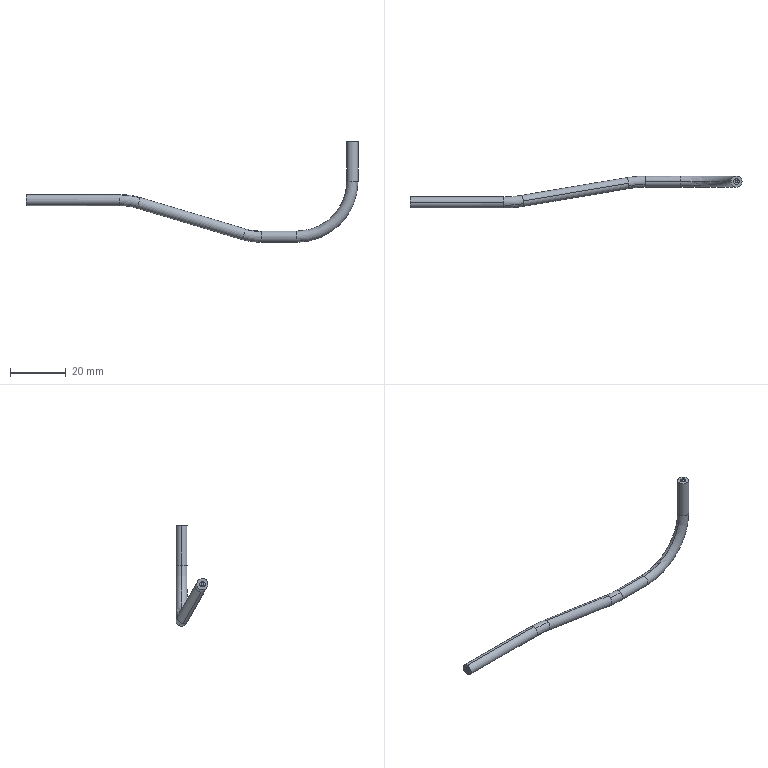Part | STEP file | [COMPANY_A Nylon 4-3 Copy] | 1 solid | 28 faces | box 119.5 x 11.5 x 36.167 mm | volume 1748 mm3 | cylinder 16 | torus 6 | plane 6 | commonest cylinder face diameters 4 x8 1 x4 2 x4
STEP:
#1=CARTESIAN_POINT('',(98.5,9.5,4.));
#2=VERTEX_POINT('',#1);
#3=CARTESIAN_POINT('',(98.5,9.5,0.));
#4=VERTEX_POINT('',#3);
#5=CARTESIAN_POINT('',(98.5,9.5,2.));
#6=DIRECTION('',(1.,0.,0.));
#7=DIRECTION('',(0.,-1.,0.));
#8=AXIS2_PLACEMENT_3D('',#5,#6,#7);
#9=CIRCLE('',#8,2.);
#10=EDGE_CURVE('',#2,#4,#9,.T.);
#11=ORIENTED_EDGE('',*,*,#10,.T.);
#12=CARTESIAN_POINT('',(120.5,9.5,22.));
#13=VERTEX_POINT('',#12);
#14=CARTESIAN_POINT('',(98.5,9.5,22.));
#15=DIRECTION('',(0.,-1.,0.));
#16=DIRECTION('',(1.,0.,0.));
#17=AXIS2_PLACEMENT_3D('',#14,#15,#16);
#18=CIRCLE('',#17,22.);
#19=EDGE_CURVE('',#4,#13,#18,.T.);
#20=ORIENTED_EDGE('',*,*,#19,.T.);
#21=CARTESIAN_POINT('',(116.5,9.5,22.));
#22=VERTEX_POINT('',#21);
#23=CARTESIAN_POINT('',(118.5,9.5,22.));
#24=DIRECTION('',(0.,0.,1.));
#25=DIRECTION('',(0.,-1.,0.));
#26=AXIS2_PLACEMENT_3D('',#23,#24,#25);
#27=CIRCLE('',#26,2.);
#28=EDGE_CURVE('',#22,#13,#27,.T.);
#29=ORIENTED_EDGE('',*,*,#28,.F.);
#30=CARTESIAN_POINT('',(98.5,9.5,22.));
#31=DIRECTION('',(0.,-1.,0.));
#32=DIRECTION('',(1.,0.,0.));
#33=AXIS2_PLACEMENT_3D('',#30,#31,#32);
#34=CIRCLE('',#33,18.);
#35=EDGE_CURVE('',#2,#22,#34,.T.);
#36=ORIENTED_EDGE('',*,*,#35,.F.);
#37=EDGE_LOOP('',(#11,#20,#29,#36));
#38=FACE_OUTER_BOUND('',#37,.T.);
#39=CARTESIAN_POINT('',(98.5,9.5,22.));
#40=DIRECTION('',(0.,-1.,0.));
#41=DIRECTION('',(-1.,0.,0.));
#42=AXIS2_PLACEMENT_3D('',#39,#40,#41);
#43=TOROIDAL_SURFACE('',#42,20.,2.);
#44=ADVANCED_FACE('',(#38),#43,.T.);
#45=CARTESIAN_POINT('',(78.559,8.964,1.024));
#46=VERTEX_POINT('',#45);
#47=CARTESIAN_POINT('',(78.481,9.9,1.297));
#48=VERTEX_POINT('',#47);
#49=CARTESIAN_POINT('',(79.131,8.964,2.941));
#50=DIRECTION('',(0.9458,0.1607,-0.2821));
#51=DIRECTION('',(0.,-0.8689,-0.4949));
#52=AXIS2_PLACEMENT_3D('',#49,#50,#51);
#53=CIRCLE('',#52,2.);
#54=EDGE_CURVE('',#46,#48,#53,.T.);
#55=ORIENTED_EDGE('',*,*,#54,.T.);
#56=CARTESIAN_POINT('',(85.623,10.49,0.2621));
#57=VERTEX_POINT('',#56);
#58=CARTESIAN_POINT('',(85.623,-0.3987,19.379));
#59=DIRECTION('',(0.,-0.8689,-0.4949));
#60=DIRECTION('',(0.,0.4949,-0.8689));
#61=AXIS2_PLACEMENT_3D('',#58,#59,#60);
#62=CIRCLE('',#61,22.);
#63=EDGE_CURVE('',#48,#57,#62,.T.);
#64=ORIENTED_EDGE('',*,*,#63,.T.);
#65=CARTESIAN_POINT('',(85.623,9.5,0.));
#66=VERTEX_POINT('',#65);
#67=CARTESIAN_POINT('',(85.623,9.5,2.));
#68=DIRECTION('',(1.,0.,0.));
#69=DIRECTION('',(0.,-0.8689,-0.4949));
#70=AXIS2_PLACEMENT_3D('',#67,#68,#69);
#71=CIRCLE('',#70,2.);
#72=EDGE_CURVE('',#66,#57,#71,.T.);
#73=ORIENTED_EDGE('',*,*,#72,.F.);
#74=CARTESIAN_POINT('',(85.623,8.51,3.738));
#75=VERTEX_POINT('',#74);
#76=CARTESIAN_POINT('',(85.623,9.5,2.));
#77=DIRECTION('',(1.,0.,0.));
#78=DIRECTION('',(0.,-0.8689,-0.4949));
#79=AXIS2_PLACEMENT_3D('',#76,#77,#78);
#80=CIRCLE('',#79,2.);
#81=EDGE_CURVE('',#75,#66,#80,.T.);
#82=ORIENTED_EDGE('',*,*,#81,.F.);
#83=CARTESIAN_POINT('',(79.78,8.028,4.585));
#84=VERTEX_POINT('',#83);
#85=CARTESIAN_POINT('',(85.623,-0.3987,19.379));
#86=DIRECTION('',(0.,-0.8689,-0.4949));
#87=DIRECTION('',(0.,0.4949,-0.8689));
#88=AXIS2_PLACEMENT_3D('',#85,#86,#87);
#89=CIRCLE('',#88,18.);
#90=EDGE_CURVE('',#84,#75,#89,.T.);
#91=ORIENTED_EDGE('',*,*,#90,.F.);
#92=CARTESIAN_POINT('',(79.131,8.964,2.941));
#93=DIRECTION('',(0.9458,0.1607,-0.2821));
#94=DIRECTION('',(0.,-0.8689,-0.4949));
#95=AXIS2_PLACEMENT_3D('',#92,#93,#94);
#96=CIRCLE('',#95,2.);
#97=EDGE_CURVE('',#84,#46,#96,.T.);
#98=ORIENTED_EDGE('',*,*,#97,.T.);
#99=EDGE_LOOP('',(#55,#64,#73,#82,#91,#98));
#100=FACE_OUTER_BOUND('',#99,.T.);
#101=CARTESIAN_POINT('',(85.623,-0.3987,19.379));
#102=DIRECTION('',(0.,-0.8689,-0.4949));
#103=DIRECTION('',(0.,-0.4949,0.8689));
#104=AXIS2_PLACEMENT_3D('',#101,#102,#103);
#105=TOROIDAL_SURFACE('',#104,20.,2.);
#106=ADVANCED_FACE('',(#100),#105,.T.);
#107=CARTESIAN_POINT('',(41.937,1.6,15.87));
#108=VERTEX_POINT('',#107);
#109=CARTESIAN_POINT('',(40.716,2.536,12.31));
#110=VERTEX_POINT('',#109);
#111=CARTESIAN_POINT('',(41.288,2.536,14.226));
#112=DIRECTION('',(0.9458,0.1607,-0.2821));
#113=DIRECTION('',(0.2858,0.,0.9583));
#114=AXIS2_PLACEMENT_3D('',#111,#112,#113);
#115=CIRCLE('',#114,2.);
#116=EDGE_CURVE('',#108,#110,#115,.T.);
#117=ORIENTED_EDGE('',*,*,#116,.F.);
#118=CARTESIAN_POINT('',(34.796,1.01,16.905));
#119=VERTEX_POINT('',#118);
#120=CARTESIAN_POINT('',(34.796,11.899,-2.211));
#121=DIRECTION('',(0.,-0.8689,-0.4949));
#122=DIRECTION('',(0.,0.4949,-0.8689));
#123=AXIS2_PLACEMENT_3D('',#120,#121,#122);
#124=CIRCLE('',#123,22.);
#125=EDGE_CURVE('',#108,#119,#124,.T.);
#126=ORIENTED_EDGE('',*,*,#125,.T.);
#127=CARTESIAN_POINT('',(34.796,2.,13.167));
#128=VERTEX_POINT('',#127);
#129=CARTESIAN_POINT('',(34.796,2.,15.167));
#130=DIRECTION('',(-1.,0.,0.));
#131=DIRECTION('',(0.,-0.8689,-0.4949));
#132=AXIS2_PLACEMENT_3D('',#129,#130,#131);
#133=CIRCLE('',#132,2.);
#134=EDGE_CURVE('',#128,#119,#133,.T.);
#135=ORIENTED_EDGE('',*,*,#134,.F.);
#136=CARTESIAN_POINT('',(34.796,2.99,13.429));
#137=VERTEX_POINT('',#136);
#138=CARTESIAN_POINT('',(34.796,2.,15.167));
#139=DIRECTION('',(-1.,0.,0.));
#140=DIRECTION('',(0.,-0.8689,-0.4949));
#141=AXIS2_PLACEMENT_3D('',#138,#139,#140);
#142=CIRCLE('',#141,2.);
#143=EDGE_CURVE('',#137,#128,#142,.T.);
#144=ORIENTED_EDGE('',*,*,#143,.F.);
#145=CARTESIAN_POINT('',(40.639,3.472,12.582));
#146=VERTEX_POINT('',#145);
#147=CARTESIAN_POINT('',(34.796,11.899,-2.211));
#148=DIRECTION('',(0.,-0.8689,-0.4949));
#149=DIRECTION('',(0.,0.4949,-0.8689));
#150=AXIS2_PLACEMENT_3D('',#147,#148,#149);
#151=CIRCLE('',#150,18.);
#152=EDGE_CURVE('',#146,#137,#151,.T.);
#153=ORIENTED_EDGE('',*,*,#152,.F.);
#154=CARTESIAN_POINT('',(41.288,2.536,14.226));
#155=DIRECTION('',(0.9458,0.1607,-0.2821));
#156=DIRECTION('',(0.2858,0.,0.9583));
#157=AXIS2_PLACEMENT_3D('',#154,#155,#156);
#158=CIRCLE('',#157,2.);
#159=EDGE_CURVE('',#110,#146,#158,.T.);
#160=ORIENTED_EDGE('',*,*,#159,.F.);
#161=EDGE_LOOP('',(#117,#126,#135,#144,#153,#160));
#162=FACE_OUTER_BOUND('',#161,.T.);
#163=CARTESIAN_POINT('',(34.796,11.899,-2.211));
#164=DIRECTION('',(0.,-0.8689,-0.4949));
#165=DIRECTION('',(0.,0.4949,-0.8689));
#166=AXIS2_PLACEMENT_3D('',#163,#164,#165);
#167=TOROIDAL_SURFACE('',#166,20.,2.);
#168=ADVANCED_FACE('',(#162),#167,.T.);
#169=CARTESIAN_POINT('',(1.,1.5,15.167));
#170=VERTEX_POINT('',#169);
#171=CARTESIAN_POINT('',(1.,2.5,15.167));
#172=VERTEX_POINT('',#171);
#173=CARTESIAN_POINT('',(1.,2.,15.167));
#174=DIRECTION('',(-1.,0.,0.));
#175=DIRECTION('',(0.,0.,-1.));
#176=AXIS2_PLACEMENT_3D('',#173,#174,#175);
#177=CIRCLE('',#176,0.5);
#178=EDGE_CURVE('',#170,#172,#177,.T.);
#179=ORIENTED_EDGE('',*,*,#178,.F.);
#180=CARTESIAN_POINT('',(18.,1.5,15.167));
#181=VERTEX_POINT('',#180);
#182=CARTESIAN_POINT('',(0.,1.5,15.167));
#183=DIRECTION('',(1.,0.,0.));
#184=VECTOR('',#183,1000.);
#185=LINE('',#182,#184);
#186=EDGE_CURVE('',#170,#181,#185,.T.);
#187=ORIENTED_EDGE('',*,*,#186,.T.);
#188=CARTESIAN_POINT('',(18.,2.5,15.167));
#189=VERTEX_POINT('',#188);
#190=CARTESIAN_POINT('',(18.,2.,15.167));
#191=DIRECTION('',(-1.,0.,0.));
#192=DIRECTION('',(0.,-1.,0.));
#193=AXIS2_PLACEMENT_3D('',#190,#191,#192);
#194=CIRCLE('',#193,0.5);
#195=EDGE_CURVE('',#181,#189,#194,.T.);
#196=ORIENTED_EDGE('',*,*,#195,.T.);
#197=CARTESIAN_POINT('',(0.,2.5,15.167));
#198=DIRECTION('',(1.,0.,0.));
#199=VECTOR('',#198,1000.);
#200=LINE('',#197,#199);
#201=EDGE_CURVE('',#172,#189,#200,.T.);
#202=ORIENTED_EDGE('',*,*,#201,.F.);
#203=EDGE_LOOP('',(#179,#187,#196,#202));
#204=FACE_OUTER_BOUND('',#203,.T.);
#205=CARTESIAN_POINT('',(0.,2.,15.167));
#206=DIRECTION('',(1.,0.,0.));
#207=DIRECTION('',(0.,1.,0.));
#208=AXIS2_PLACEMENT_3D('',#205,#206,#207);
#209=CYLINDRICAL_SURFACE('',#208,0.5);
#210=ADVANCED_FACE('',(#204),#209,.T.);
#211=CARTESIAN_POINT('',(1.,2.,14.167));
#212=VERTEX_POINT('',#211);
#213=CARTESIAN_POINT('',(1.,2.,16.167));
#214=VERTEX_POINT('',#213);
#215=CARTESIAN_POINT('',(1.,2.,15.167));
#216=DIRECTION('',(1.,0.,0.));
#217=DIRECTION('',(0.,0.,1.));
#218=AXIS2_PLACEMENT_3D('',#215,#216,#217);
#219=CIRCLE('',#218,1.);
#220=EDGE_CURVE('',#212,#214,#219,.T.);
#221=ORIENTED_EDGE('',*,*,#220,.F.);
#222=CARTESIAN_POINT('',(18.,2.,14.167));
#223=VERTEX_POINT('',#222);
#224=CARTESIAN_POINT('',(1.,2.,14.167));
#225=DIRECTION('',(1.,0.,0.));
#226=VECTOR('',#225,1000.);
#227=LINE('',#224,#226);
#228=EDGE_CURVE('',#212,#223,#227,.T.);
#229=ORIENTED_EDGE('',*,*,#228,.T.);
#230=CARTESIAN_POINT('',(18.,2.,16.167));
#231=VERTEX_POINT('',#230);
#232=CARTESIAN_POINT('',(18.,2.,15.167));
#233=DIRECTION('',(-1.,0.,0.));
#234=DIRECTION('',(0.,0.,-1.));
#235=AXIS2_PLACEMENT_3D('',#232,#233,#234);
#236=CIRCLE('',#235,1.);
#237=EDGE_CURVE('',#231,#223,#236,.T.);
#238=ORIENTED_EDGE('',*,*,#237,.F.);
#239=CARTESIAN_POINT('',(1.,2.,16.167));
#240=DIRECTION('',(1.,0.,0.));
#241=VECTOR('',#240,1000.);
#242=LINE('',#239,#241);
#243=EDGE_CURVE('',#214,#231,#242,.T.);
#244=ORIENTED_EDGE('',*,*,#243,.F.);
#245=EDGE_LOOP('',(#221,#229,#238,#244));
#246=FACE_OUTER_BOUND('',#245,.T.);
#247=CARTESIAN_POINT('',(1.,2.,15.167));
#248=DIRECTION('',(1.,0.,0.));
#249=DIRECTION('',(0.,0.,1.));
#250=AXIS2_PLACEMENT_3D('',#247,#248,#249);
#251=CYLINDRICAL_SURFACE('',#250,1.);
#252=ADVANCED_FACE('',(#246),#251,.F.);
#253=CARTESIAN_POINT('',(118.5,9.,36.167));
#254=VERTEX_POINT('',#253);
#255=CARTESIAN_POINT('',(118.5,10.,36.167));
#256=VERTEX_POINT('',#255);
#257=CARTESIAN_POINT('',(118.5,9.5,36.167));
#258=DIRECTION('',(0.,0.,1.));
#259=DIRECTION('',(-1.,0.,0.));
#260=AXIS2_PLACEMENT_3D('',#257,#258,#259);
#261=CIRCLE('',#260,0.5);
#262=EDGE_CURVE('',#254,#256,#261,.T.);
#263=ORIENTED_EDGE('',*,*,#262,.F.);
#264=CARTESIAN_POINT('',(118.5,9.,19.167));
#265=VERTEX_POINT('',#264);
#266=CARTESIAN_POINT('',(118.5,9.,37.167));
#267=DIRECTION('',(0.,0.,-1.));
#268=VECTOR('',#267,1000.);
#269=LINE('',#266,#268);
#270=EDGE_CURVE('',#254,#265,#269,.T.);
#271=ORIENTED_EDGE('',*,*,#270,.T.);
#272=CARTESIAN_POINT('',(118.5,10.,19.167));
#273=VERTEX_POINT('',#272);
#274=CARTESIAN_POINT('',(118.5,9.5,19.167));
#275=DIRECTION('',(0.,0.,1.));
#276=DIRECTION('',(0.,-1.,0.));
#277=AXIS2_PLACEMENT_3D('',#274,#275,#276);
#278=CIRCLE('',#277,0.5);
#279=EDGE_CURVE('',#265,#273,#278,.T.);
#280=ORIENTED_EDGE('',*,*,#279,.T.);
#281=CARTESIAN_POINT('',(118.5,10.,37.167));
#282=DIRECTION('',(0.,0.,-1.));
#283=VECTOR('',#282,1000.);
#284=LINE('',#281,#283);
#285=EDGE_CURVE('',#256,#273,#284,.T.);
#286=ORIENTED_EDGE('',*,*,#285,.F.);
#287=EDGE_LOOP('',(#263,#271,#280,#286));
#288=FACE_OUTER_BOUND('',#287,.T.);
#289=CARTESIAN_POINT('',(118.5,9.5,37.167));
#290=DIRECTION('',(0.,0.,-1.));
#291=DIRECTION('',(0.,1.,0.));
#292=AXIS2_PLACEMENT_3D('',#289,#290,#291);
#293=CYLINDRICAL_SURFACE('',#292,0.5);
#294=ADVANCED_FACE('',(#288),#293,.T.);
#295=CARTESIAN_POINT('',(117.5,9.5,36.167));
#296=VERTEX_POINT('',#295);
#297=CARTESIAN_POINT('',(119.5,9.5,36.167));
#298=VERTEX_POINT('',#297);
#299=CARTESIAN_POINT('',(118.5,9.5,36.167));
#300=DIRECTION('',(0.,0.,-1.));
#301=DIRECTION('',(1.,0.,0.));
#302=AXIS2_PLACEMENT_3D('',#299,#300,#301);
#303=CIRCLE('',#302,1.);
#304=EDGE_CURVE('',#296,#298,#303,.T.);
#305=ORIENTED_EDGE('',*,*,#304,.F.);
#306=CARTESIAN_POINT('',(117.5,9.5,19.167));
#307=VERTEX_POINT('',#306);
#308=CARTESIAN_POINT('',(117.5,9.5,36.167));
#309=DIRECTION('',(0.,0.,-1.));
#310=VECTOR('',#309,1000.);
#311=LINE('',#308,#310);
#312=EDGE_CURVE('',#296,#307,#311,.T.);
#313=ORIENTED_EDGE('',*,*,#312,.T.);
#314=CARTESIAN_POINT('',(119.5,9.5,19.167));
#315=VERTEX_POINT('',#314);
#316=CARTESIAN_POINT('',(118.5,9.5,19.167));
#317=DIRECTION('',(0.,0.,1.));
#318=DIRECTION('',(-1.,0.,0.));
#319=AXIS2_PLACEMENT_3D('',#316,#317,#318);
#320=CIRCLE('',#319,1.);
#321=EDGE_CURVE('',#315,#307,#320,.T.);
#322=ORIENTED_EDGE('',*,*,#321,.F.);
#323=CARTESIAN_POINT('',(119.5,9.5,36.167));
#324=DIRECTION('',(0.,0.,-1.));
#325=VECTOR('',#324,1000.);
#326=LINE('',#323,#325);
#327=EDGE_CURVE('',#298,#315,#326,.T.);
#328=ORIENTED_EDGE('',*,*,#327,.F.);
#329=EDGE_LOOP('',(#305,#313,#322,#328));
#330=FACE_OUTER_BOUND('',#329,.T.);
#331=CARTESIAN_POINT('',(118.5,9.5,36.167));
#332=DIRECTION('',(0.,0.,-1.));
#333=DIRECTION('',(1.,0.,0.));
#334=AXIS2_PLACEMENT_3D('',#331,#332,#333);
#335=CYLINDRICAL_SURFACE('',#334,1.);
#336=ADVANCED_FACE('',(#330),#335,.F.);
#337=CARTESIAN_POINT('',(85.623,9.5,4.));
#338=VERTEX_POINT('',#337);
#339=CARTESIAN_POINT('',(85.623,9.5,2.));
#340=DIRECTION('',(1.,0.,0.));
#341=DIRECTION('',(0.,-0.8689,-0.4949));
#342=AXIS2_PLACEMENT_3D('',#339,#340,#341);
#343=CIRCLE('',#342,2.);
#344=EDGE_CURVE('',#338,#75,#343,.T.);
#345=ORIENTED_EDGE('',*,*,#344,.T.);
#346=ORIENTED_EDGE('',*,*,#81,.T.);
#347=CARTESIAN_POINT('',(85.623,9.5,0.));
#348=DIRECTION('',(1.,0.,0.));
#349=VECTOR('',#348,1000.);
#350=LINE('',#347,#349);
#351=EDGE_CURVE('',#66,#4,#350,.T.);
#352=ORIENTED_EDGE('',*,*,#351,.T.);
#353=ORIENTED_EDGE('',*,*,#10,.F.);
#354=CARTESIAN_POINT('',(85.623,9.5,4.));
#355=DIRECTION('',(1.,0.,0.));
#356=VECTOR('',#355,1000.);
#357=LINE('',#354,#356);
#358=EDGE_CURVE('',#338,#2,#357,.T.);
#359=ORIENTED_EDGE('',*,*,#358,.F.);
#360=EDGE_LOOP('',(#345,#346,#352,#353,#359));
#361=FACE_OUTER_BOUND('',#360,.T.);
#362=CARTESIAN_POINT('',(85.623,9.5,2.));
#363=DIRECTION('',(1.,0.,0.));
#364=DIRECTION('',(0.,0.,1.));
#365=AXIS2_PLACEMENT_3D('',#362,#363,#364);
#366=CYLINDRICAL_SURFACE('',#365,2.);
#367=ADVANCED_FACE('',(#361),#366,.T.);
#368=CARTESIAN_POINT('',(41.859,2.536,16.143));
#369=VERTEX_POINT('',#368);
#370=CARTESIAN_POINT('',(41.288,2.536,14.226));
#371=DIRECTION('',(0.9458,0.1607,-0.2821));
#372=DIRECTION('',(0.2858,0.,0.9583));
#373=AXIS2_PLACEMENT_3D('',#370,#371,#372);
#374=CIRCLE('',#373,2.);
#375=EDGE_CURVE('',#369,#108,#374,.T.);
#376=ORIENTED_EDGE('',*,*,#375,.T.);
#377=ORIENTED_EDGE('',*,*,#116,.T.);
#378=CARTESIAN_POINT('',(40.716,2.536,12.31));
#379=DIRECTION('',(0.9458,0.1607,-0.2821));
#380=VECTOR('',#379,1000.);
#381=LINE('',#378,#380);
#382=EDGE_CURVE('',#110,#46,#381,.T.);
#383=ORIENTED_EDGE('',*,*,#382,.T.);
#384=ORIENTED_EDGE('',*,*,#97,.F.);
#385=CARTESIAN_POINT('',(79.702,8.964,4.858));
#386=VERTEX_POINT('',#385);
#387=CARTESIAN_POINT('',(79.131,8.964,2.941));
#388=DIRECTION('',(0.9458,0.1607,-0.2821));
#389=DIRECTION('',(0.,-0.8689,-0.4949));
#390=AXIS2_PLACEMENT_3D('',#387,#388,#389);
#391=CIRCLE('',#390,2.);
#392=EDGE_CURVE('',#386,#84,#391,.T.);
#393=ORIENTED_EDGE('',*,*,#392,.F.);
#394=CARTESIAN_POINT('',(41.859,2.536,16.143));
#395=DIRECTION('',(0.9458,0.1607,-0.2821));
#396=VECTOR('',#395,1000.);
#397=LINE('',#394,#396);
#398=EDGE_CURVE('',#369,#386,#397,.T.);
#399=ORIENTED_EDGE('',*,*,#398,.F.);
#400=EDGE_LOOP('',(#376,#377,#383,#384,#393,#399));
#401=FACE_OUTER_BOUND('',#400,.T.);
#402=CARTESIAN_POINT('',(41.288,2.536,14.226));
#403=DIRECTION('',(0.9458,0.1607,-0.2821));
#404=DIRECTION('',(0.2858,0.,0.9583));
#405=AXIS2_PLACEMENT_3D('',#402,#403,#404);
#406=CYLINDRICAL_SURFACE('',#405,2.);
#407=ADVANCED_FACE('',(#401),#406,.T.);
#408=ORIENTED_EDGE('',*,*,#28,.T.);
#409=CARTESIAN_POINT('',(120.5,9.5,36.167));
#410=VERTEX_POINT('',#409);
#411=CARTESIAN_POINT('',(120.5,9.5,22.));
#412=DIRECTION('',(0.,0.,1.));
#413=VECTOR('',#412,1000.);
#414=LINE('',#411,#413);
#415=EDGE_CURVE('',#13,#410,#414,.T.);
#416=ORIENTED_EDGE('',*,*,#415,.T.);
#417=CARTESIAN_POINT('',(116.5,9.5,36.167));
#418=VERTEX_POINT('',#417);
#419=CARTESIAN_POINT('',(118.5,9.5,36.167));
#420=DIRECTION('',(0.,0.,-1.));
#421=DIRECTION('',(1.,0.,0.));
#422=AXIS2_PLACEMENT_3D('',#419,#420,#421);
#423=CIRCLE('',#422,2.);
#424=EDGE_CURVE('',#410,#418,#423,.T.);
#425=ORIENTED_EDGE('',*,*,#424,.T.);
#426=CARTESIAN_POINT('',(116.5,9.5,22.));
#427=DIRECTION('',(0.,0.,1.));
#428=VECTOR('',#427,1000.);
#429=LINE('',#426,#428);
#430=EDGE_CURVE('',#22,#418,#429,.T.);
#431=ORIENTED_EDGE('',*,*,#430,.F.);
#432=EDGE_LOOP('',(#408,#416,#425,#431));
#433=FACE_OUTER_BOUND('',#432,.T.);
#434=CARTESIAN_POINT('',(118.5,9.5,22.));
#435=DIRECTION('',(0.,0.,1.));
#436=DIRECTION('',(-1.,0.,0.));
#437=AXIS2_PLACEMENT_3D('',#434,#435,#436);
#438=CYLINDRICAL_SURFACE('',#437,2.);
#439=ADVANCED_FACE('',(#433),#438,.T.);
#440=ORIENTED_EDGE('',*,*,#134,.T.);
#441=CARTESIAN_POINT('',(34.796,2.,17.167));
#442=VERTEX_POINT('',#441);
#443=CARTESIAN_POINT('',(34.796,2.,15.167));
#444=DIRECTION('',(-1.,0.,0.));
#445=DIRECTION('',(0.,-0.8689,-0.4949));
#446=AXIS2_PLACEMENT_3D('',#443,#444,#445);
#447=CIRCLE('',#446,2.);
#448=EDGE_CURVE('',#119,#442,#447,.T.);
#449=ORIENTED_EDGE('',*,*,#448,.T.);
#450=CARTESIAN_POINT('',(1.,2.,17.167));
#451=VERTEX_POINT('',#450);
#452=CARTESIAN_POINT('',(34.796,2.,17.167));
#453=DIRECTION('',(-1.,0.,0.));
#454=VECTOR('',#453,1000.);
#455=LINE('',#452,#454);
#456=EDGE_CURVE('',#442,#451,#455,.T.);
#457=ORIENTED_EDGE('',*,*,#456,.T.);
#458=CARTESIAN_POINT('',(1.,2.,13.167));
#459=VERTEX_POINT('',#458);
#460=CARTESIAN_POINT('',(1.,2.,15.167));
#461=DIRECTION('',(1.,0.,0.));
#462=DIRECTION('',(0.,0.,1.));
#463=AXIS2_PLACEMENT_3D('',#460,#461,#462);
#464=CIRCLE('',#463,2.);
#465=EDGE_CURVE('',#451,#459,#464,.T.);
#466=ORIENTED_EDGE('',*,*,#465,.T.);
#467=CARTESIAN_POINT('',(34.796,2.,13.167));
#468=DIRECTION('',(-1.,0.,0.));
#469=VECTOR('',#468,1000.);
#470=LINE('',#467,#469);
#471=EDGE_CURVE('',#128,#459,#470,.T.);
#472=ORIENTED_EDGE('',*,*,#471,.F.);
#473=EDGE_LOOP('',(#440,#449,#457,#466,#472));
#474=FACE_OUTER_BOUND('',#473,.T.);
#475=CARTESIAN_POINT('',(34.796,2.,15.167));
#476=DIRECTION('',(-1.,0.,0.));
#477=DIRECTION('',(0.,0.,-1.));
#478=AXIS2_PLACEMENT_3D('',#475,#476,#477);
#479=CYLINDRICAL_SURFACE('',#478,2.);
#480=ADVANCED_FACE('',(#474),#479,.T.);
#481=CARTESIAN_POINT('',(1.,2.,15.167));
#482=DIRECTION('',(1.,0.,0.));
#483=DIRECTION('',(0.,0.,1.));
#484=AXIS2_PLACEMENT_3D('',#481,#482,#483);
#485=CIRCLE('',#484,1.);
#486=EDGE_CURVE('',#214,#212,#485,.T.);
#487=ORIENTED_EDGE('',*,*,#486,.T.);
#488=ORIENTED_EDGE('',*,*,#220,.T.);
#489=EDGE_LOOP('',(#487,#488));
#490=FACE_BOUND('',#489,.T.);
#491=CARTESIAN_POINT('',(1.,2.,15.167));
#492=DIRECTION('',(1.,0.,0.));
#493=DIRECTION('',(0.,0.,1.));
#494=AXIS2_PLACEMENT_3D('',#491,#492,#493);
#495=CIRCLE('',#494,2.);
#496=EDGE_CURVE('',#459,#451,#495,.T.);
#497=ORIENTED_EDGE('',*,*,#496,.F.);
#498=ORIENTED_EDGE('',*,*,#465,.F.);
#499=EDGE_LOOP('',(#497,#498));
#500=FACE_OUTER_BOUND('',#499,.T.);
#501=CARTESIAN_POINT('',(1.,2.,15.167));
#502=DIRECTION('',(-1.,0.,0.));
#503=DIRECTION('',(0.,0.,-1.));
#504=AXIS2_PLACEMENT_3D('',#501,#502,#503);
#505=PLANE('',#504);
#506=ADVANCED_FACE('',(#490,#500),#505,.T.);
#507=ORIENTED_EDGE('',*,*,#456,.F.);
#508=CARTESIAN_POINT('',(34.796,2.,15.167));
#509=DIRECTION('',(-1.,0.,0.));
#510=DIRECTION('',(0.,-0.8689,-0.4949));
#511=AXIS2_PLACEMENT_3D('',#508,#509,#510);
#512=CIRCLE('',#511,2.);
#513=EDGE_CURVE('',#442,#137,#512,.T.);
#514=ORIENTED_EDGE('',*,*,#513,.T.);
#515=ORIENTED_EDGE('',*,*,#143,.T.);
#516=ORIENTED_EDGE('',*,*,#471,.T.);
#517=ORIENTED_EDGE('',*,*,#496,.T.);
#518=EDGE_LOOP('',(#507,#514,#515,#516,#517));
#519=FACE_OUTER_BOUND('',#518,.T.);
#520=CARTESIAN_POINT('',(34.796,2.,15.167));
#521=DIRECTION('',(-1.,0.,0.));
#522=DIRECTION('',(0.,0.,-1.));
#523=AXIS2_PLACEMENT_3D('',#520,#521,#522);
#524=CYLINDRICAL_SURFACE('',#523,2.);
#525=ADVANCED_FACE('',(#519),#524,.T.);
#526=CARTESIAN_POINT('',(118.5,9.5,36.167));
#527=DIRECTION('',(0.,0.,-1.));
#528=DIRECTION('',(1.,0.,0.));
#529=AXIS2_PLACEMENT_3D('',#526,#527,#528);
#530=CIRCLE('',#529,1.);
#531=EDGE_CURVE('',#298,#296,#530,.T.);
#532=ORIENTED_EDGE('',*,*,#531,.T.);
#533=ORIENTED_EDGE('',*,*,#304,.T.);
#534=EDGE_LOOP('',(#532,#533));
#535=FACE_BOUND('',#534,.T.);
#536=CARTESIAN_POINT('',(118.5,9.5,36.167));
#537=DIRECTION('',(0.,0.,-1.));
#538=DIRECTION('',(1.,0.,0.));
#539=AXIS2_PLACEMENT_3D('',#536,#537,#538);
#540=CIRCLE('',#539,2.);
#541=EDGE_CURVE('',#418,#410,#540,.T.);
#542=ORIENTED_EDGE('',*,*,#541,.F.);
#543=ORIENTED_EDGE('',*,*,#424,.F.);
#544=EDGE_LOOP('',(#542,#543));
#545=FACE_OUTER_BOUND('',#544,.T.);
#546=CARTESIAN_POINT('',(118.5,9.5,36.167));
#547=DIRECTION('',(0.,0.,1.));
#548=DIRECTION('',(-1.,0.,0.));
#549=AXIS2_PLACEMENT_3D('',#546,#547,#548);
#550=PLANE('',#549);
#551=ADVANCED_FACE('',(#535,#545),#550,.T.);
#552=ORIENTED_EDGE('',*,*,#415,.F.);
#553=CARTESIAN_POINT('',(118.5,9.5,22.));
#554=DIRECTION('',(0.,0.,1.));
#555=DIRECTION('',(0.,-1.,0.));
#556=AXIS2_PLACEMENT_3D('',#553,#554,#555);
#557=CIRCLE('',#556,2.);
#558=EDGE_CURVE('',#13,#22,#557,.T.);
#559=ORIENTED_EDGE('',*,*,#558,.T.);
#560=ORIENTED_EDGE('',*,*,#430,.T.);
#561=ORIENTED_EDGE('',*,*,#541,.T.);
#562=EDGE_LOOP('',(#552,#559,#560,#561));
#563=FACE_OUTER_BOUND('',#562,.T.);
#564=CARTESIAN_POINT('',(118.5,9.5,22.));
#565=DIRECTION('',(0.,0.,1.));
#566=DIRECTION('',(-1.,0.,0.));
#567=AXIS2_PLACEMENT_3D('',#564,#565,#566);
#568=CYLINDRICAL_SURFACE('',#567,2.);
#569=ADVANCED_FACE('',(#563),#568,.T.);
#570=ORIENTED_EDGE('',*,*,#125,.F.);
#571=ORIENTED_EDGE('',*,*,#375,.F.);
#572=CARTESIAN_POINT('',(41.288,2.536,14.226));
#573=DIRECTION('',(0.9458,0.1607,-0.2821));
#574=DIRECTION('',(0.2858,0.,0.9583));
#575=AXIS2_PLACEMENT_3D('',#572,#573,#574);
#576=CIRCLE('',#575,2.);
#577=EDGE_CURVE('',#146,#369,#576,.T.);
#578=ORIENTED_EDGE('',*,*,#577,.F.);
#579=ORIENTED_EDGE('',*,*,#152,.T.);
#580=ORIENTED_EDGE('',*,*,#513,.F.);
#581=ORIENTED_EDGE('',*,*,#448,.F.);
#582=EDGE_LOOP('',(#570,#571,#578,#579,#580,#581));
#583=FACE_OUTER_BOUND('',#582,.T.);
#584=CARTESIAN_POINT('',(34.796,11.899,-2.211));
#585=DIRECTION('',(0.,-0.8689,-0.4949));
#586=DIRECTION('',(0.,0.4949,-0.8689));
#587=AXIS2_PLACEMENT_3D('',#584,#585,#586);
#588=TOROIDAL_SURFACE('',#587,20.,2.);
#589=ADVANCED_FACE('',(#583),#588,.T.);
#590=ORIENTED_EDGE('',*,*,#382,.F.);
#591=ORIENTED_EDGE('',*,*,#159,.T.);
#592=ORIENTED_EDGE('',*,*,#577,.T.);
#593=ORIENTED_EDGE('',*,*,#398,.T.);
#594=CARTESIAN_POINT('',(79.131,8.964,2.941));
#595=DIRECTION('',(0.9458,0.1607,-0.2821));
#596=DIRECTION('',(0.,-0.8689,-0.4949));
#597=AXIS2_PLACEMENT_3D('',#594,#595,#596);
#598=CIRCLE('',#597,2.);
#599=EDGE_CURVE('',#48,#386,#598,.T.);
#600=ORIENTED_EDGE('',*,*,#599,.F.);
#601=ORIENTED_EDGE('',*,*,#54,.F.);
#602=EDGE_LOOP('',(#590,#591,#592,#593,#600,#601));
#603=FACE_OUTER_BOUND('',#602,.T.);
#604=CARTESIAN_POINT('',(41.288,2.536,14.226));
#605=DIRECTION('',(0.9458,0.1607,-0.2821));
#606=DIRECTION('',(0.2858,0.,0.9583));
#607=AXIS2_PLACEMENT_3D('',#604,#605,#606);
#608=CYLINDRICAL_SURFACE('',#607,2.);
#609=ADVANCED_FACE('',(#603),#608,.T.);
#610=ORIENTED_EDGE('',*,*,#63,.F.);
#611=ORIENTED_EDGE('',*,*,#599,.T.);
#612=ORIENTED_EDGE('',*,*,#392,.T.);
#613=ORIENTED_EDGE('',*,*,#90,.T.);
#614=ORIENTED_EDGE('',*,*,#344,.F.);
#615=CARTESIAN_POINT('',(85.623,9.5,2.));
#616=DIRECTION('',(1.,0.,0.));
#617=DIRECTION('',(0.,-0.8689,-0.4949));
#618=AXIS2_PLACEMENT_3D('',#615,#616,#617);
#619=CIRCLE('',#618,2.);
#620=EDGE_CURVE('',#57,#338,#619,.T.);
#621=ORIENTED_EDGE('',*,*,#620,.F.);
#622=EDGE_LOOP('',(#610,#611,#612,#613,#614,#621));
#623=FACE_OUTER_BOUND('',#622,.T.);
#624=CARTESIAN_POINT('',(85.623,-0.3987,19.379));
#625=DIRECTION('',(0.,-0.8689,-0.4949));
#626=DIRECTION('',(0.,-0.4949,0.8689));
#627=AXIS2_PLACEMENT_3D('',#624,#625,#626);
#628=TOROIDAL_SURFACE('',#627,20.,2.);
#629=ADVANCED_FACE('',(#623),#628,.T.);
#630=ORIENTED_EDGE('',*,*,#351,.F.);
#631=ORIENTED_EDGE('',*,*,#72,.T.);
#632=ORIENTED_EDGE('',*,*,#620,.T.);
#633=ORIENTED_EDGE('',*,*,#358,.T.);
#634=CARTESIAN_POINT('',(98.5,9.5,2.));
#635=DIRECTION('',(1.,0.,0.));
#636=DIRECTION('',(0.,-1.,0.));
#637=AXIS2_PLACEMENT_3D('',#634,#635,#636);
#638=CIRCLE('',#637,2.);
#639=EDGE_CURVE('',#4,#2,#638,.T.);
#640=ORIENTED_EDGE('',*,*,#639,.F.);
#641=EDGE_LOOP('',(#630,#631,#632,#633,#640));
#642=FACE_OUTER_BOUND('',#641,.T.);
#643=CARTESIAN_POINT('',(85.623,9.5,2.));
#644=DIRECTION('',(1.,0.,0.));
#645=DIRECTION('',(0.,0.,1.));
#646=AXIS2_PLACEMENT_3D('',#643,#644,#645);
#647=CYLINDRICAL_SURFACE('',#646,2.);
#648=ADVANCED_FACE('',(#642),#647,.T.);
#649=ORIENTED_EDGE('',*,*,#19,.F.);
#650=ORIENTED_EDGE('',*,*,#639,.T.);
#651=ORIENTED_EDGE('',*,*,#35,.T.);
#652=ORIENTED_EDGE('',*,*,#558,.F.);
#653=EDGE_LOOP('',(#649,#650,#651,#652));
#654=FACE_OUTER_BOUND('',#653,.T.);
#655=CARTESIAN_POINT('',(98.5,9.5,22.));
#656=DIRECTION('',(0.,-1.,0.));
#657=DIRECTION('',(-1.,0.,0.));
#658=AXIS2_PLACEMENT_3D('',#655,#656,#657);
#659=TOROIDAL_SURFACE('',#658,20.,2.);
#660=ADVANCED_FACE('',(#654),#659,.T.);
#661=CARTESIAN_POINT('',(118.5,9.5,19.167));
#662=DIRECTION('',(0.,0.,1.));
#663=DIRECTION('',(0.,-1.,0.));
#664=AXIS2_PLACEMENT_3D('',#661,#662,#663);
#665=CIRCLE('',#664,0.5);
#666=EDGE_CURVE('',#273,#265,#665,.T.);
#667=ORIENTED_EDGE('',*,*,#666,.F.);
#668=ORIENTED_EDGE('',*,*,#279,.F.);
#669=EDGE_LOOP('',(#667,#668));
#670=FACE_BOUND('',#669,.T.);
#671=ORIENTED_EDGE('',*,*,#321,.T.);
#672=CARTESIAN_POINT('',(118.5,9.5,19.167));
#673=DIRECTION('',(0.,0.,1.));
#674=DIRECTION('',(-1.,0.,0.));
#675=AXIS2_PLACEMENT_3D('',#672,#673,#674);
#676=CIRCLE('',#675,1.);
#677=EDGE_CURVE('',#307,#315,#676,.T.);
#678=ORIENTED_EDGE('',*,*,#677,.T.);
#679=EDGE_LOOP('',(#671,#678));
#680=FACE_OUTER_BOUND('',#679,.T.);
#681=CARTESIAN_POINT('',(118.5,9.5,19.167));
#682=DIRECTION('',(0.,0.,-1.));
#683=DIRECTION('',(1.,0.,0.));
#684=AXIS2_PLACEMENT_3D('',#681,#682,#683);
#685=PLANE('',#684);
#686=ADVANCED_FACE('',(#670,#680),#685,.F.);
#687=ORIENTED_EDGE('',*,*,#312,.F.);
#688=ORIENTED_EDGE('',*,*,#531,.F.);
#689=ORIENTED_EDGE('',*,*,#327,.T.);
#690=ORIENTED_EDGE('',*,*,#677,.F.);
#691=EDGE_LOOP('',(#687,#688,#689,#690));
#692=FACE_OUTER_BOUND('',#691,.T.);
#693=CARTESIAN_POINT('',(118.5,9.5,36.167));
#694=DIRECTION('',(0.,0.,-1.));
#695=DIRECTION('',(1.,0.,0.));
#696=AXIS2_PLACEMENT_3D('',#693,#694,#695);
#697=CYLINDRICAL_SURFACE('',#696,1.);
#698=ADVANCED_FACE('',(#692),#697,.F.);
#699=ORIENTED_EDGE('',*,*,#270,.F.);
#700=CARTESIAN_POINT('',(118.5,9.5,36.167));
#701=DIRECTION('',(0.,0.,1.));
#702=DIRECTION('',(-1.,0.,0.));
#703=AXIS2_PLACEMENT_3D('',#700,#701,#702);
#704=CIRCLE('',#703,0.5);
#705=EDGE_CURVE('',#256,#254,#704,.T.);
#706=ORIENTED_EDGE('',*,*,#705,.F.);
#707=ORIENTED_EDGE('',*,*,#285,.T.);
#708=ORIENTED_EDGE('',*,*,#666,.T.);
#709=EDGE_LOOP('',(#699,#706,#707,#708));
#710=FACE_OUTER_BOUND('',#709,.T.);
#711=CARTESIAN_POINT('',(118.5,9.5,37.167));
#712=DIRECTION('',(0.,0.,-1.));
#713=DIRECTION('',(0.,1.,0.));
#714=AXIS2_PLACEMENT_3D('',#711,#712,#713);
#715=CYLINDRICAL_SURFACE('',#714,0.5);
#716=ADVANCED_FACE('',(#710),#715,.T.);
#717=ORIENTED_EDGE('',*,*,#705,.T.);
#718=ORIENTED_EDGE('',*,*,#262,.T.);
#719=EDGE_LOOP('',(#717,#718));
#720=FACE_OUTER_BOUND('',#719,.T.);
#721=CARTESIAN_POINT('',(118.5,9.5,36.167));
#722=DIRECTION('',(0.,0.,1.));
#723=DIRECTION('',(-1.,0.,0.));
#724=AXIS2_PLACEMENT_3D('',#721,#722,#723);
#725=PLANE('',#724);
#726=ADVANCED_FACE('',(#720),#725,.T.);
#727=CARTESIAN_POINT('',(18.,2.,15.167));
#728=DIRECTION('',(-1.,0.,0.));
#729=DIRECTION('',(0.,-1.,0.));
#730=AXIS2_PLACEMENT_3D('',#727,#728,#729);
#731=CIRCLE('',#730,0.5);
#732=EDGE_CURVE('',#189,#181,#731,.T.);
#733=ORIENTED_EDGE('',*,*,#732,.F.);
#734=ORIENTED_EDGE('',*,*,#195,.F.);
#735=EDGE_LOOP('',(#733,#734));
#736=FACE_BOUND('',#735,.T.);
#737=ORIENTED_EDGE('',*,*,#237,.T.);
#738=CARTESIAN_POINT('',(18.,2.,15.167));
#739=DIRECTION('',(-1.,0.,0.));
#740=DIRECTION('',(0.,0.,-1.));
#741=AXIS2_PLACEMENT_3D('',#738,#739,#740);
#742=CIRCLE('',#741,1.);
#743=EDGE_CURVE('',#223,#231,#742,.T.);
#744=ORIENTED_EDGE('',*,*,#743,.T.);
#745=EDGE_LOOP('',(#737,#744));
#746=FACE_OUTER_BOUND('',#745,.T.);
#747=CARTESIAN_POINT('',(18.,2.,15.167));
#748=DIRECTION('',(1.,0.,0.));
#749=DIRECTION('',(0.,0.,1.));
#750=AXIS2_PLACEMENT_3D('',#747,#748,#749);
#751=PLANE('',#750);
#752=ADVANCED_FACE('',(#736,#746),#751,.F.);
#753=ORIENTED_EDGE('',*,*,#228,.F.);
#754=ORIENTED_EDGE('',*,*,#486,.F.);
#755=ORIENTED_EDGE('',*,*,#243,.T.);
#756=ORIENTED_EDGE('',*,*,#743,.F.);
#757=EDGE_LOOP('',(#753,#754,#755,#756));
#758=FACE_OUTER_BOUND('',#757,.T.);
#759=CARTESIAN_POINT('',(1.,2.,15.167));
#760=DIRECTION('',(1.,0.,0.));
#761=DIRECTION('',(0.,0.,1.));
#762=AXIS2_PLACEMENT_3D('',#759,#760,#761);
#763=CYLINDRICAL_SURFACE('',#762,1.);
#764=ADVANCED_FACE('',(#758),#763,.F.);
#765=ORIENTED_EDGE('',*,*,#186,.F.);
#766=CARTESIAN_POINT('',(1.,2.,15.167));
#767=DIRECTION('',(-1.,0.,0.));
#768=DIRECTION('',(0.,0.,-1.));
#769=AXIS2_PLACEMENT_3D('',#766,#767,#768);
#770=CIRCLE('',#769,0.5);
#771=EDGE_CURVE('',#172,#170,#770,.T.);
#772=ORIENTED_EDGE('',*,*,#771,.F.);
#773=ORIENTED_EDGE('',*,*,#201,.T.);
#774=ORIENTED_EDGE('',*,*,#732,.T.);
#775=EDGE_LOOP('',(#765,#772,#773,#774));
#776=FACE_OUTER_BOUND('',#775,.T.);
#777=CARTESIAN_POINT('',(0.,2.,15.167));
#778=DIRECTION('',(1.,0.,0.));
#779=DIRECTION('',(0.,1.,0.));
#780=AXIS2_PLACEMENT_3D('',#777,#778,#779);
#781=CYLINDRICAL_SURFACE('',#780,0.5);
#782=ADVANCED_FACE('',(#776),#781,.T.);
#783=ORIENTED_EDGE('',*,*,#771,.T.);
#784=ORIENTED_EDGE('',*,*,#178,.T.);
#785=EDGE_LOOP('',(#783,#784));
#786=FACE_OUTER_BOUND('',#785,.T.);
#787=CARTESIAN_POINT('',(1.,2.,15.167));
#788=DIRECTION('',(-1.,0.,0.));
#789=DIRECTION('',(0.,0.,-1.));
#790=AXIS2_PLACEMENT_3D('',#787,#788,#789);
#791=PLANE('',#790);
#792=ADVANCED_FACE('',(#786),#791,.T.);
#793=CLOSED_SHELL('',(#44,#106,#168,#210,#252,#294,#336,#367,#407,#439,#480,#506,#525,#551,#569,#589,#609,#629,#648,#660,#686,#698,#716,#726,#752,#764,#782,#792));
#794=MANIFOLD_SOLID_BREP('',#793);
#795=CARTESIAN_POINT('',(0.,0.,0.));
#796=DIRECTION('',(0.,0.,1.));
#797=DIRECTION('',(1.,0.,0.));
#798=AXIS2_PLACEMENT_3D('',#795,#796,#797);
#799=(LENGTH_UNIT()NAMED_UNIT(*)SI_UNIT(.MILLI.,.METRE.));
#800=UNCERTAINTY_MEASURE_WITH_UNIT(LENGTH_MEASURE(0.00001),#799,'','');
#801=(NAMED_UNIT(*)PLANE_ANGLE_UNIT()SI_UNIT($,.RADIAN.));
#802=(NAMED_UNIT(*)SI_UNIT($,.STERADIAN.)SOLID_ANGLE_UNIT());
#803=(GEOMETRIC_REPRESENTATION_CONTEXT(3)GLOBAL_UNCERTAINTY_ASSIGNED_CONTEXT((#800))GLOBAL_UNIT_ASSIGNED_CONTEXT((#799,#801,#802))REPRESENTATION_CONTEXT('',''));
#804=ADVANCED_BREP_SHAPE_REPRESENTATION('',(#794,#798),#803);